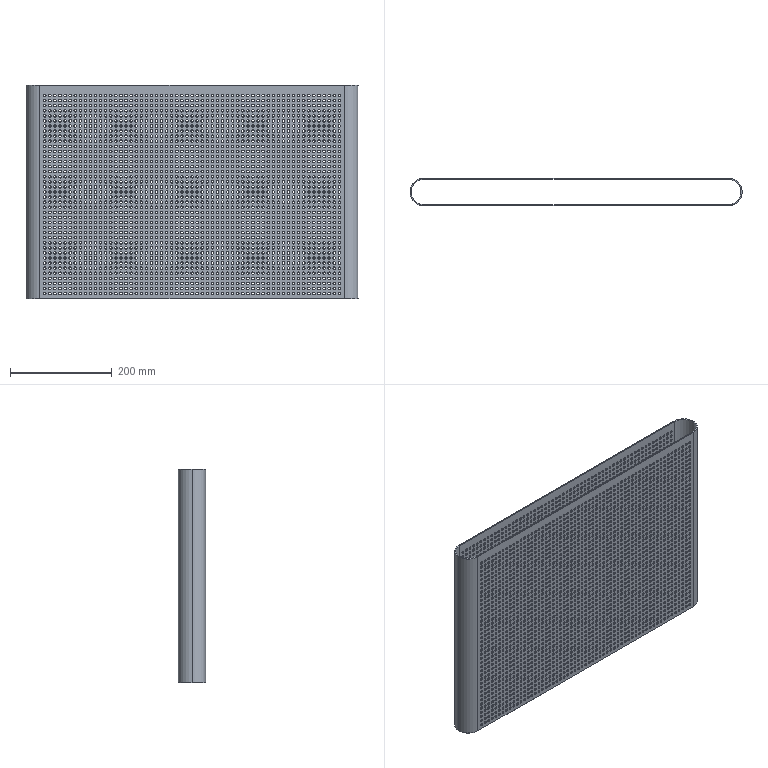Part | SolidWorks | features LPattern 2, Extrusion 1, ICE 1 | 1 solid | 9452 faces | volume 959871 mm3 | cylinder 9446 | plane 6 | commonest cylinder face diameters 5 x9440 50 x3 54 x3